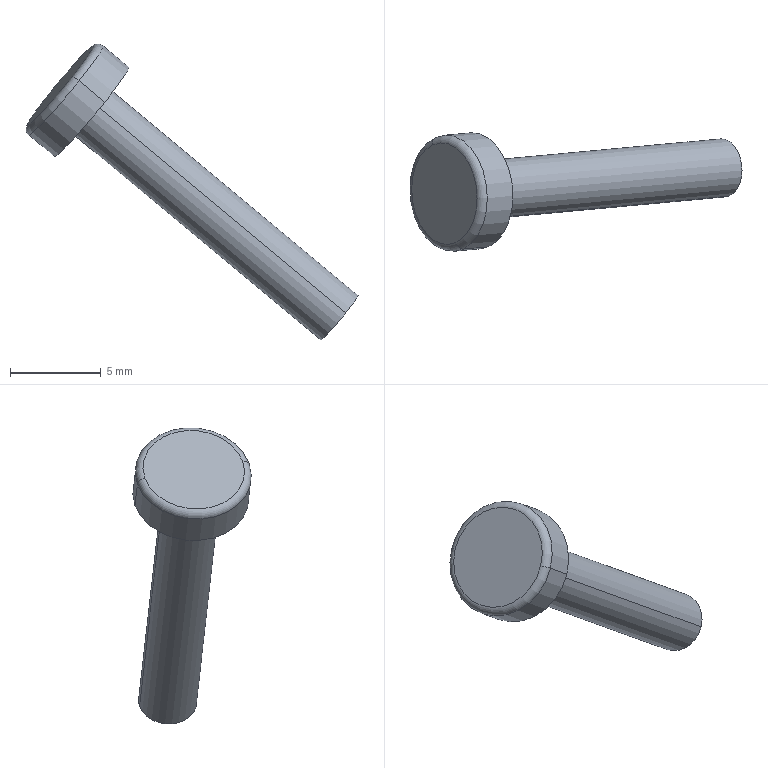Part | SolidWorks | features SplitBody 1 | 1 solid | 9 faces | box 18.257 x 6.517 x 16.285 mm | volume 214.224 mm3 | cylinder 4 | plane 3 | torus 2 | commonest cylinder face diameters 3.2 x2 6.4 x2
STEP:
#1=CARTESIAN_POINT('',(518.443,292.699,-337.518));
#2=VERTEX_POINT('',#1);
#3=CARTESIAN_POINT('',(519.714,287.324,-336.596));
#4=VERTEX_POINT('',#3);
#5=CARTESIAN_POINT('',(519.079,290.012,-337.057));
#6=DIRECTION('',(-0.767,-0.07213,0.6375));
#7=DIRECTION('',(0.227,-0.9599,0.1646));
#8=AXIS2_PLACEMENT_3D('',#5,#6,#7);
#9=CIRCLE('',#8,2.8);
#10=EDGE_CURVE('',#2,#4,#9,.T.);
#11=ORIENTED_EDGE('',*,*,#10,.F.);
#12=CARTESIAN_POINT('',(518.659,293.112,-337.839));
#13=VERTEX_POINT('',#12);
#14=CARTESIAN_POINT('',(518.75,292.728,-337.773));
#15=DIRECTION('',(-0.6001,-0.271,-0.7527));
#16=DIRECTION('',(-0.7819,0.,0.6234));
#17=AXIS2_PLACEMENT_3D('',#14,#15,#16);
#18=CIRCLE('',#17,0.4);
#19=EDGE_CURVE('',#2,#13,#18,.T.);
#20=ORIENTED_EDGE('',*,*,#19,.T.);
#21=CARTESIAN_POINT('',(520.112,286.969,-336.786));
#22=VERTEX_POINT('',#21);
#23=CARTESIAN_POINT('',(519.385,290.041,-337.312));
#24=DIRECTION('',(0.767,0.07213,-0.6375));
#25=DIRECTION('',(0.227,-0.9599,0.1646));
#26=AXIS2_PLACEMENT_3D('',#23,#24,#25);
#27=CIRCLE('',#26,3.2);
#28=EDGE_CURVE('',#22,#13,#27,.T.);
#29=ORIENTED_EDGE('',*,*,#28,.F.);
#30=CARTESIAN_POINT('',(520.021,287.353,-336.851));
#31=DIRECTION('',(0.6001,0.271,0.7527));
#32=DIRECTION('',(0.7819,0.,-0.6234));
#33=AXIS2_PLACEMENT_3D('',#30,#31,#32);
#34=CIRCLE('',#33,0.4);
#35=EDGE_CURVE('',#4,#22,#34,.T.);
#36=ORIENTED_EDGE('',*,*,#35,.F.);
#37=EDGE_LOOP('',(#11,#20,#29,#36));
#38=FACE_OUTER_BOUND('',#37,.T.);
#39=CARTESIAN_POINT('',(519.385,290.041,-337.312));
#40=DIRECTION('',(0.767,0.07213,-0.6375));
#41=DIRECTION('',(0.227,-0.9599,0.1646));
#42=AXIS2_PLACEMENT_3D('',#39,#40,#41);
#43=TOROIDAL_SURFACE('',#42,2.8,0.4);
#44=ADVANCED_FACE('',(#38),#43,.T.);
#45=CARTESIAN_POINT('',(534.783,289.919,-349.544));
#46=VERTEX_POINT('',#45);
#47=CARTESIAN_POINT('',(534.056,292.99,-350.071));
#48=VERTEX_POINT('',#47);
#49=CARTESIAN_POINT('',(534.42,291.454,-349.808));
#50=DIRECTION('',(0.767,0.07213,-0.6375));
#51=DIRECTION('',(0.227,-0.9599,0.1646));
#52=AXIS2_PLACEMENT_3D('',#49,#50,#51);
#53=CIRCLE('',#52,1.6);
#54=EDGE_CURVE('',#46,#48,#53,.T.);
#55=ORIENTED_EDGE('',*,*,#54,.F.);
#56=CARTESIAN_POINT('',(521.16,288.637,-338.222));
#57=VERTEX_POINT('',#56);
#58=CARTESIAN_POINT('',(534.783,289.919,-349.544));
#59=DIRECTION('',(-0.767,-0.07213,0.6375));
#60=VECTOR('',#59,1000.);
#61=LINE('',#58,#60);
#62=EDGE_CURVE('',#46,#57,#61,.T.);
#63=ORIENTED_EDGE('',*,*,#62,.T.);
#64=CARTESIAN_POINT('',(520.434,291.709,-338.749));
#65=VERTEX_POINT('',#64);
#66=CARTESIAN_POINT('',(520.797,290.173,-338.485));
#67=DIRECTION('',(0.767,0.07213,-0.6375));
#68=DIRECTION('',(0.227,-0.9599,0.1646));
#69=AXIS2_PLACEMENT_3D('',#66,#67,#68);
#70=CIRCLE('',#69,1.6);
#71=EDGE_CURVE('',#57,#65,#70,.T.);
#72=ORIENTED_EDGE('',*,*,#71,.T.);
#73=CARTESIAN_POINT('',(534.056,292.99,-350.071));
#74=DIRECTION('',(-0.767,-0.07213,0.6375));
#75=VECTOR('',#74,1000.);
#76=LINE('',#73,#75);
#77=EDGE_CURVE('',#48,#65,#76,.T.);
#78=ORIENTED_EDGE('',*,*,#77,.F.);
#79=EDGE_LOOP('',(#55,#63,#72,#78));
#80=FACE_OUTER_BOUND('',#79,.T.);
#81=CARTESIAN_POINT('',(534.42,291.454,-349.808));
#82=DIRECTION('',(-0.767,-0.07213,0.6375));
#83=DIRECTION('',(-0.227,0.9599,-0.1646));
#84=AXIS2_PLACEMENT_3D('',#81,#82,#83);
#85=CYLINDRICAL_SURFACE('',#84,1.6);
#86=ADVANCED_FACE('',(#80),#85,.T.);
#87=CARTESIAN_POINT('',(521.523,287.102,-337.959));
#88=VERTEX_POINT('',#87);
#89=CARTESIAN_POINT('',(520.07,293.245,-339.012));
#90=VERTEX_POINT('',#89);
#91=CARTESIAN_POINT('',(520.797,290.173,-338.485));
#92=DIRECTION('',(0.767,0.07213,-0.6375));
#93=DIRECTION('',(0.227,-0.9599,0.1646));
#94=AXIS2_PLACEMENT_3D('',#91,#92,#93);
#95=CIRCLE('',#94,3.2);
#96=EDGE_CURVE('',#88,#90,#95,.T.);
#97=ORIENTED_EDGE('',*,*,#96,.F.);
#98=CARTESIAN_POINT('',(521.523,287.102,-337.959));
#99=DIRECTION('',(-0.767,-0.07213,0.6375));
#100=VECTOR('',#99,1000.);
#101=LINE('',#98,#100);
#102=EDGE_CURVE('',#88,#22,#101,.T.);
#103=ORIENTED_EDGE('',*,*,#102,.T.);
#104=ORIENTED_EDGE('',*,*,#28,.T.);
#105=CARTESIAN_POINT('',(520.07,293.245,-339.012));
#106=DIRECTION('',(-0.767,-0.07213,0.6375));
#107=VECTOR('',#106,1000.);
#108=LINE('',#105,#107);
#109=EDGE_CURVE('',#90,#13,#108,.T.);
#110=ORIENTED_EDGE('',*,*,#109,.F.);
#111=EDGE_LOOP('',(#97,#103,#104,#110));
#112=FACE_OUTER_BOUND('',#111,.T.);
#113=CARTESIAN_POINT('',(520.797,290.173,-338.485));
#114=DIRECTION('',(-0.767,-0.07213,0.6375));
#115=DIRECTION('',(-0.227,0.9599,-0.1646));
#116=AXIS2_PLACEMENT_3D('',#113,#114,#115);
#117=CYLINDRICAL_SURFACE('',#116,3.2);
#118=ADVANCED_FACE('',(#112),#117,.T.);
#119=ORIENTED_EDGE('',*,*,#102,.F.);
#120=CARTESIAN_POINT('',(520.797,290.173,-338.485));
#121=DIRECTION('',(0.767,0.07213,-0.6375));
#122=DIRECTION('',(0.227,-0.9599,0.1646));
#123=AXIS2_PLACEMENT_3D('',#120,#121,#122);
#124=CIRCLE('',#123,3.2);
#125=EDGE_CURVE('',#90,#88,#124,.T.);
#126=ORIENTED_EDGE('',*,*,#125,.F.);
#127=ORIENTED_EDGE('',*,*,#109,.T.);
#128=CARTESIAN_POINT('',(519.385,290.041,-337.312));
#129=DIRECTION('',(0.767,0.07213,-0.6375));
#130=DIRECTION('',(0.227,-0.9599,0.1646));
#131=AXIS2_PLACEMENT_3D('',#128,#129,#130);
#132=CIRCLE('',#131,3.2);
#133=EDGE_CURVE('',#13,#22,#132,.T.);
#134=ORIENTED_EDGE('',*,*,#133,.T.);
#135=EDGE_LOOP('',(#119,#126,#127,#134));
#136=FACE_OUTER_BOUND('',#135,.T.);
#137=CARTESIAN_POINT('',(520.797,290.173,-338.485));
#138=DIRECTION('',(-0.767,-0.07213,0.6375));
#139=DIRECTION('',(-0.227,0.9599,-0.1646));
#140=AXIS2_PLACEMENT_3D('',#137,#138,#139);
#141=CYLINDRICAL_SURFACE('',#140,3.2);
#142=ADVANCED_FACE('',(#136),#141,.T.);
#143=CARTESIAN_POINT('',(519.079,290.012,-337.057));
#144=DIRECTION('',(-0.767,-0.07213,0.6375));
#145=DIRECTION('',(0.227,-0.9599,0.1646));
#146=AXIS2_PLACEMENT_3D('',#143,#144,#145);
#147=CIRCLE('',#146,2.8);
#148=EDGE_CURVE('',#4,#2,#147,.T.);
#149=ORIENTED_EDGE('',*,*,#148,.T.);
#150=ORIENTED_EDGE('',*,*,#10,.T.);
#151=EDGE_LOOP('',(#149,#150));
#152=FACE_OUTER_BOUND('',#151,.T.);
#153=CARTESIAN_POINT('',(519.079,290.012,-337.057));
#154=DIRECTION('',(0.767,0.07213,-0.6375));
#155=DIRECTION('',(0.227,-0.9599,0.1646));
#156=AXIS2_PLACEMENT_3D('',#153,#154,#155);
#157=PLANE('',#156);
#158=ADVANCED_FACE('',(#152),#157,.F.);
#159=CARTESIAN_POINT('',(520.797,290.173,-338.485));
#160=DIRECTION('',(0.767,0.07213,-0.6375));
#161=DIRECTION('',(0.227,-0.9599,0.1646));
#162=AXIS2_PLACEMENT_3D('',#159,#160,#161);
#163=CIRCLE('',#162,1.6);
#164=EDGE_CURVE('',#65,#57,#163,.T.);
#165=ORIENTED_EDGE('',*,*,#164,.F.);
#166=ORIENTED_EDGE('',*,*,#71,.F.);
#167=EDGE_LOOP('',(#165,#166));
#168=FACE_BOUND('',#167,.T.);
#169=ORIENTED_EDGE('',*,*,#125,.T.);
#170=ORIENTED_EDGE('',*,*,#96,.T.);
#171=EDGE_LOOP('',(#169,#170));
#172=FACE_OUTER_BOUND('',#171,.T.);
#173=CARTESIAN_POINT('',(520.797,290.173,-338.485));
#174=DIRECTION('',(0.767,0.07213,-0.6375));
#175=DIRECTION('',(0.227,-0.9599,0.1646));
#176=AXIS2_PLACEMENT_3D('',#173,#174,#175);
#177=PLANE('',#176);
#178=ADVANCED_FACE('',(#168,#172),#177,.T.);
#179=ORIENTED_EDGE('',*,*,#62,.F.);
#180=CARTESIAN_POINT('',(534.42,291.454,-349.808));
#181=DIRECTION('',(0.767,0.07213,-0.6375));
#182=DIRECTION('',(0.227,-0.9599,0.1646));
#183=AXIS2_PLACEMENT_3D('',#180,#181,#182);
#184=CIRCLE('',#183,1.6);
#185=EDGE_CURVE('',#48,#46,#184,.T.);
#186=ORIENTED_EDGE('',*,*,#185,.F.);
#187=ORIENTED_EDGE('',*,*,#77,.T.);
#188=ORIENTED_EDGE('',*,*,#164,.T.);
#189=EDGE_LOOP('',(#179,#186,#187,#188));
#190=FACE_OUTER_BOUND('',#189,.T.);
#191=CARTESIAN_POINT('',(534.42,291.454,-349.808));
#192=DIRECTION('',(-0.767,-0.07213,0.6375));
#193=DIRECTION('',(-0.227,0.9599,-0.1646));
#194=AXIS2_PLACEMENT_3D('',#191,#192,#193);
#195=CYLINDRICAL_SURFACE('',#194,1.6);
#196=ADVANCED_FACE('',(#190),#195,.T.);
#197=ORIENTED_EDGE('',*,*,#185,.T.);
#198=ORIENTED_EDGE('',*,*,#54,.T.);
#199=EDGE_LOOP('',(#197,#198));
#200=FACE_OUTER_BOUND('',#199,.T.);
#201=CARTESIAN_POINT('',(534.42,291.454,-349.808));
#202=DIRECTION('',(0.767,0.07213,-0.6375));
#203=DIRECTION('',(0.227,-0.9599,0.1646));
#204=AXIS2_PLACEMENT_3D('',#201,#202,#203);
#205=PLANE('',#204);
#206=ADVANCED_FACE('',(#200),#205,.T.);
#207=ORIENTED_EDGE('',*,*,#19,.F.);
#208=ORIENTED_EDGE('',*,*,#148,.F.);
#209=ORIENTED_EDGE('',*,*,#35,.T.);
#210=ORIENTED_EDGE('',*,*,#133,.F.);
#211=EDGE_LOOP('',(#207,#208,#209,#210));
#212=FACE_OUTER_BOUND('',#211,.T.);
#213=CARTESIAN_POINT('',(519.385,290.041,-337.312));
#214=DIRECTION('',(0.767,0.07213,-0.6375));
#215=DIRECTION('',(0.227,-0.9599,0.1646));
#216=AXIS2_PLACEMENT_3D('',#213,#214,#215);
#217=TOROIDAL_SURFACE('',#216,2.8,0.4);
#218=ADVANCED_FACE('',(#212),#217,.T.);
#219=CLOSED_SHELL('',(#44,#86,#118,#142,#158,#178,#196,#206,#218));
#220=MANIFOLD_SOLID_BREP('',#219);
#221=CARTESIAN_POINT('',(0.,0.,0.));
#222=DIRECTION('',(0.,0.,1.));
#223=DIRECTION('',(1.,0.,0.));
#224=AXIS2_PLACEMENT_3D('',#221,#222,#223);
#225=(LENGTH_UNIT()NAMED_UNIT(*)SI_UNIT(.MILLI.,.METRE.));
#226=UNCERTAINTY_MEASURE_WITH_UNIT(LENGTH_MEASURE(0.00001),#225,'','');
#227=(NAMED_UNIT(*)PLANE_ANGLE_UNIT()SI_UNIT($,.RADIAN.));
#228=(NAMED_UNIT(*)SI_UNIT($,.STERADIAN.)SOLID_ANGLE_UNIT());
#229=(GEOMETRIC_REPRESENTATION_CONTEXT(3)GLOBAL_UNCERTAINTY_ASSIGNED_CONTEXT((#226))GLOBAL_UNIT_ASSIGNED_CONTEXT((#225,#227,#228))REPRESENTATION_CONTEXT('',''));
#230=ADVANCED_BREP_SHAPE_REPRESENTATION('',(#220,#224),#229);